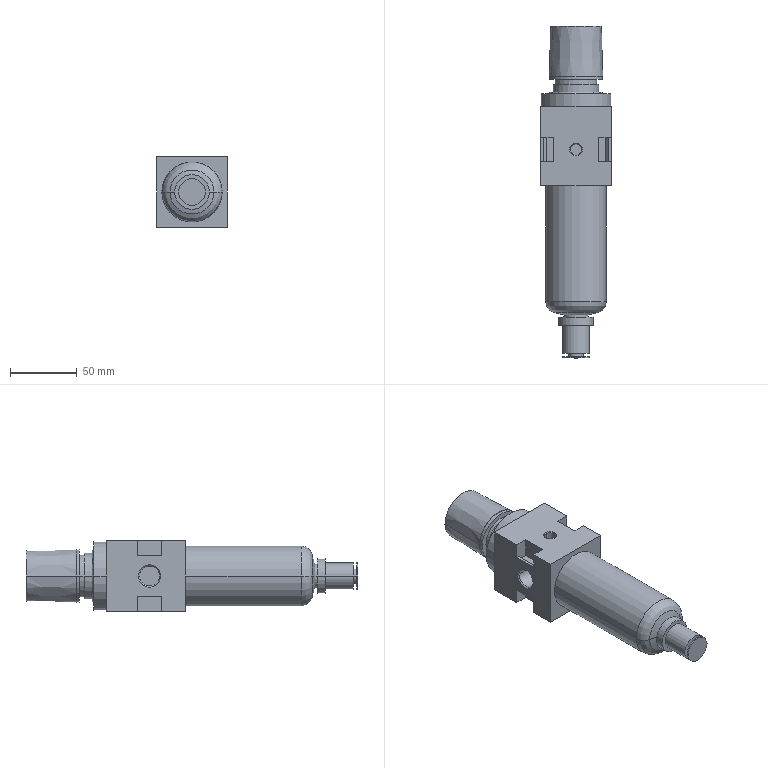Part | NX | 1 solid | 89 faces | box 53 x 248.5 x 53 mm | volume 389353 mm3 | plane 45 | cylinder 28 | cone 14 | torus 2 | commonest cylinder face diameters 8.57 x4 14.95 x4 20 x4 11 x2 18 x2 26 x2